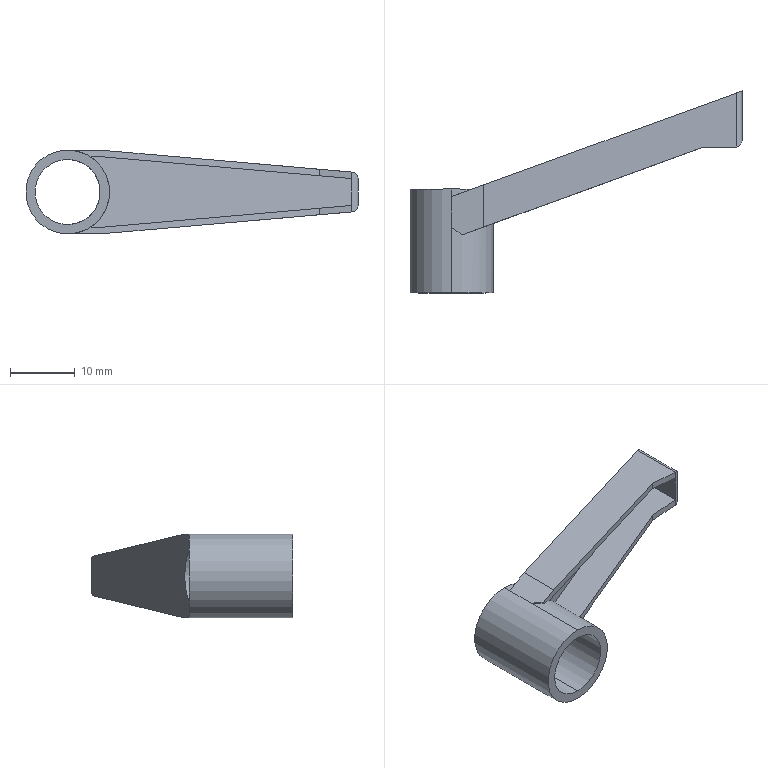Part | SolidWorks | features BaseBody 1, Shell 1 | 1 solid | 33 faces | box 51.5 x 31.3 x 13 mm | volume 1733 mm3 | plane 23 | cylinder 10 | commonest cylinder face diameters 13 x4 2 x3 10.1 x2 12.1 x1
STEP:
#1=CARTESIAN_POINT('',(3.238,20.3,5.636));
#2=VERTEX_POINT('',#1);
#3=CARTESIAN_POINT('',(0.,20.3,6.5));
#4=VERTEX_POINT('',#3);
#5=CARTESIAN_POINT('',(0.,20.3,0.));
#6=DIRECTION('',(0.,-1.,0.));
#7=DIRECTION('',(0.,0.,-1.));
#8=AXIS2_PLACEMENT_3D('',#5,#6,#7);
#9=CIRCLE('',#8,6.5);
#10=EDGE_CURVE('',#2,#4,#9,.T.);
#11=ORIENTED_EDGE('',*,*,#10,.T.);
#12=CARTESIAN_POINT('',(0.,19.121,6.5));
#13=VERTEX_POINT('',#12);
#14=CARTESIAN_POINT('',(0.,12.25,6.5));
#15=DIRECTION('',(0.,-1.,0.));
#16=VECTOR('',#15,1000.);
#17=LINE('',#14,#16);
#18=EDGE_CURVE('',#4,#13,#17,.T.);
#19=ORIENTED_EDGE('',*,*,#18,.T.);
#20=CARTESIAN_POINT('',(3.238,20.3,5.636));
#21=CARTESIAN_POINT('',(2.247,19.939,6.205));
#22=CARTESIAN_POINT('',(1.143,19.537,6.5));
#23=CARTESIAN_POINT('',(0.,19.121,6.5));
#24=(BOUNDED_CURVE()B_SPLINE_CURVE(3,(#20,#21,#22,#23),.UNSPECIFIED.,.F.,.F.)B_SPLINE_CURVE_WITH_KNOTS((4,4),(4.191,4.712),.UNSPECIFIED.)CURVE()GEOMETRIC_REPRESENTATION_ITEM()RATIONAL_B_SPLINE_CURVE((1.,0.9775,0.9775,1.))REPRESENTATION_ITEM(''));
#25=EDGE_CURVE('',#2,#13,#24,.T.);
#26=ORIENTED_EDGE('',*,*,#25,.F.);
#27=EDGE_LOOP('',(#11,#19,#26));
#28=FACE_OUTER_BOUND('',#27,.T.);
#29=CARTESIAN_POINT('',(0.,12.25,0.));
#30=DIRECTION('',(0.,-1.,0.));
#31=DIRECTION('',(0.,0.,-1.));
#32=AXIS2_PLACEMENT_3D('',#29,#30,#31);
#33=CYLINDRICAL_SURFACE('',#32,6.5);
#34=ADVANCED_FACE('',(#28),#33,.T.);
#35=CARTESIAN_POINT('',(1.638,13.2,6.29));
#36=VERTEX_POINT('',#35);
#37=CARTESIAN_POINT('',(0.,14.347,6.5));
#38=VERTEX_POINT('',#37);
#39=CARTESIAN_POINT('',(1.638,13.2,6.29));
#40=CARTESIAN_POINT('',(1.103,13.575,6.43));
#41=CARTESIAN_POINT('',(0.5536,13.959,6.5));
#42=CARTESIAN_POINT('',(0.,14.347,6.5));
#43=(BOUNDED_CURVE()B_SPLINE_CURVE(3,(#39,#40,#41,#42),.UNSPECIFIED.,.F.,.F.)B_SPLINE_CURVE_WITH_KNOTS((4,4),(1.316,1.571),.UNSPECIFIED.)CURVE()GEOMETRIC_REPRESENTATION_ITEM()RATIONAL_B_SPLINE_CURVE((1.,0.9946,0.9946,1.))REPRESENTATION_ITEM(''));
#44=EDGE_CURVE('',#36,#38,#43,.T.);
#45=ORIENTED_EDGE('',*,*,#44,.T.);
#46=CARTESIAN_POINT('',(0.,4.2,6.5));
#47=VERTEX_POINT('',#46);
#48=CARTESIAN_POINT('',(0.,12.25,6.5));
#49=DIRECTION('',(0.,-1.,0.));
#50=VECTOR('',#49,1000.);
#51=LINE('',#48,#50);
#52=EDGE_CURVE('',#38,#47,#51,.T.);
#53=ORIENTED_EDGE('',*,*,#52,.T.);
#54=CARTESIAN_POINT('',(0.,4.2,-6.5));
#55=VERTEX_POINT('',#54);
#56=CARTESIAN_POINT('',(0.,4.2,0.));
#57=DIRECTION('',(0.,1.,0.));
#58=DIRECTION('',(0.,0.,-1.));
#59=AXIS2_PLACEMENT_3D('',#56,#57,#58);
#60=CIRCLE('',#59,6.5);
#61=EDGE_CURVE('',#47,#55,#60,.T.);
#62=ORIENTED_EDGE('',*,*,#61,.T.);
#63=CARTESIAN_POINT('',(0.,14.347,-6.5));
#64=VERTEX_POINT('',#63);
#65=CARTESIAN_POINT('',(0.,12.25,-6.5));
#66=DIRECTION('',(0.,-1.,0.));
#67=VECTOR('',#66,1000.);
#68=LINE('',#65,#67);
#69=EDGE_CURVE('',#64,#55,#68,.T.);
#70=ORIENTED_EDGE('',*,*,#69,.F.);
#71=CARTESIAN_POINT('',(1.638,13.2,-6.29));
#72=VERTEX_POINT('',#71);
#73=CARTESIAN_POINT('',(0.,14.347,-6.5));
#74=CARTESIAN_POINT('',(0.5536,13.959,-6.5));
#75=CARTESIAN_POINT('',(1.103,13.575,-6.43));
#76=CARTESIAN_POINT('',(1.638,13.2,-6.29));
#77=(BOUNDED_CURVE()B_SPLINE_CURVE(3,(#73,#74,#75,#76),.UNSPECIFIED.,.F.,.T.)B_SPLINE_CURVE_WITH_KNOTS((4,4),(4.712,4.967),.UNSPECIFIED.)CURVE()GEOMETRIC_REPRESENTATION_ITEM()RATIONAL_B_SPLINE_CURVE((1.,0.9946,0.9946,1.))REPRESENTATION_ITEM(''));
#78=EDGE_CURVE('',#64,#72,#77,.T.);
#79=ORIENTED_EDGE('',*,*,#78,.T.);
#80=CARTESIAN_POINT('',(3.464,13.864,-5.5));
#81=VERTEX_POINT('',#80);
#82=CARTESIAN_POINT('',(1.638,13.2,-6.29));
#83=CARTESIAN_POINT('',(2.285,13.435,-6.122));
#84=CARTESIAN_POINT('',(2.899,13.658,-5.856));
#85=CARTESIAN_POINT('',(3.464,13.864,-5.5));
#86=(BOUNDED_CURVE()B_SPLINE_CURVE(3,(#82,#83,#84,#85),.UNSPECIFIED.,.F.,.T.)B_SPLINE_CURVE_WITH_KNOTS((4,4),(1.826,2.133),.UNSPECIFIED.)CURVE()GEOMETRIC_REPRESENTATION_ITEM()RATIONAL_B_SPLINE_CURVE((1.,0.9921,0.9921,1.))REPRESENTATION_ITEM(''));
#87=EDGE_CURVE('',#72,#81,#86,.T.);
#88=ORIENTED_EDGE('',*,*,#87,.T.);
#89=CARTESIAN_POINT('',(3.464,13.864,5.5));
#90=VERTEX_POINT('',#89);
#91=CARTESIAN_POINT('',(3.464,13.864,-5.5));
#92=CARTESIAN_POINT('',(7.97,15.504,-2.662));
#93=CARTESIAN_POINT('',(7.97,15.504,2.662));
#94=CARTESIAN_POINT('',(3.464,13.864,5.5));
#95=(BOUNDED_CURVE()B_SPLINE_CURVE(3,(#91,#92,#93,#94),.UNSPECIFIED.,.F.,.T.)B_SPLINE_CURVE_WITH_KNOTS((4,4),(2.133,4.15),.UNSPECIFIED.)CURVE()GEOMETRIC_REPRESENTATION_ITEM()RATIONAL_B_SPLINE_CURVE((1.,0.6886,0.6886,1.))REPRESENTATION_ITEM(''));
#96=EDGE_CURVE('',#81,#90,#95,.T.);
#97=ORIENTED_EDGE('',*,*,#96,.T.);
#98=CARTESIAN_POINT('',(3.464,13.864,5.5));
#99=CARTESIAN_POINT('',(2.899,13.658,5.856));
#100=CARTESIAN_POINT('',(2.285,13.435,6.122));
#101=CARTESIAN_POINT('',(1.638,13.2,6.29));
#102=(BOUNDED_CURVE()B_SPLINE_CURVE(3,(#98,#99,#100,#101),.UNSPECIFIED.,.F.,.F.)B_SPLINE_CURVE_WITH_KNOTS((4,4),(4.15,4.458),.UNSPECIFIED.)CURVE()GEOMETRIC_REPRESENTATION_ITEM()RATIONAL_B_SPLINE_CURVE((1.,0.9921,0.9921,1.))REPRESENTATION_ITEM(''));
#103=EDGE_CURVE('',#90,#36,#102,.T.);
#104=ORIENTED_EDGE('',*,*,#103,.T.);
#105=EDGE_LOOP('',(#45,#53,#62,#70,#79,#88,#97,#104));
#106=FACE_OUTER_BOUND('',#105,.T.);
#107=CARTESIAN_POINT('',(0.,12.25,0.));
#108=DIRECTION('',(0.,-1.,0.));
#109=DIRECTION('',(0.,0.,-1.));
#110=AXIS2_PLACEMENT_3D('',#107,#108,#109);
#111=CYLINDRICAL_SURFACE('',#110,6.5);
#112=ADVANCED_FACE('',(#106),#111,.T.);
#113=ORIENTED_EDGE('',*,*,#18,.F.);
#114=CARTESIAN_POINT('',(0.,20.3,-6.5));
#115=VERTEX_POINT('',#114);
#116=CARTESIAN_POINT('',(0.,20.3,0.));
#117=DIRECTION('',(0.,-1.,0.));
#118=DIRECTION('',(0.,0.,-1.));
#119=AXIS2_PLACEMENT_3D('',#116,#117,#118);
#120=CIRCLE('',#119,6.5);
#121=EDGE_CURVE('',#4,#115,#120,.T.);
#122=ORIENTED_EDGE('',*,*,#121,.T.);
#123=CARTESIAN_POINT('',(0.,19.121,-6.5));
#124=VERTEX_POINT('',#123);
#125=CARTESIAN_POINT('',(0.,12.25,-6.5));
#126=DIRECTION('',(0.,-1.,0.));
#127=VECTOR('',#126,1000.);
#128=LINE('',#125,#127);
#129=EDGE_CURVE('',#115,#124,#128,.T.);
#130=ORIENTED_EDGE('',*,*,#129,.T.);
#131=CARTESIAN_POINT('',(0.,12.25,-6.5));
#132=DIRECTION('',(0.,-1.,0.));
#133=VECTOR('',#132,1000.);
#134=LINE('',#131,#133);
#135=EDGE_CURVE('',#124,#64,#134,.T.);
#136=ORIENTED_EDGE('',*,*,#135,.T.);
#137=ORIENTED_EDGE('',*,*,#69,.T.);
#138=CARTESIAN_POINT('',(0.,4.2,0.));
#139=DIRECTION('',(0.,1.,0.));
#140=DIRECTION('',(0.,0.,-1.));
#141=AXIS2_PLACEMENT_3D('',#138,#139,#140);
#142=CIRCLE('',#141,6.5);
#143=EDGE_CURVE('',#55,#47,#142,.T.);
#144=ORIENTED_EDGE('',*,*,#143,.T.);
#145=ORIENTED_EDGE('',*,*,#52,.F.);
#146=CARTESIAN_POINT('',(0.,0.,6.5));
#147=DIRECTION('',(0.,-1.,0.));
#148=VECTOR('',#147,1000.);
#149=LINE('',#146,#148);
#150=EDGE_CURVE('',#13,#38,#149,.T.);
#151=ORIENTED_EDGE('',*,*,#150,.F.);
#152=EDGE_LOOP('',(#113,#122,#130,#136,#137,#144,#145,#151));
#153=FACE_OUTER_BOUND('',#152,.T.);
#154=CARTESIAN_POINT('',(0.,12.25,0.));
#155=DIRECTION('',(0.,-1.,0.));
#156=DIRECTION('',(0.,0.,-1.));
#157=AXIS2_PLACEMENT_3D('',#154,#155,#156);
#158=CYLINDRICAL_SURFACE('',#157,6.5);
#159=ADVANCED_FACE('',(#153),#158,.T.);
#160=CARTESIAN_POINT('',(0.,20.3,5.05));
#161=VERTEX_POINT('',#160);
#162=CARTESIAN_POINT('',(0.,20.3,-5.05));
#163=VERTEX_POINT('',#162);
#164=CARTESIAN_POINT('',(0.,20.3,0.));
#165=DIRECTION('',(0.,-1.,0.));
#166=DIRECTION('',(0.,0.,-1.));
#167=AXIS2_PLACEMENT_3D('',#164,#165,#166);
#168=CIRCLE('',#167,5.05);
#169=EDGE_CURVE('',#161,#163,#168,.T.);
#170=ORIENTED_EDGE('',*,*,#169,.F.);
#171=CARTESIAN_POINT('',(0.,4.2,5.05));
#172=VERTEX_POINT('',#171);
#173=CARTESIAN_POINT('',(0.,14.35,5.05));
#174=DIRECTION('',(0.,-1.,0.));
#175=VECTOR('',#174,1000.);
#176=LINE('',#173,#175);
#177=EDGE_CURVE('',#161,#172,#176,.T.);
#178=ORIENTED_EDGE('',*,*,#177,.T.);
#179=CARTESIAN_POINT('',(0.,4.2,-5.05));
#180=VERTEX_POINT('',#179);
#181=CARTESIAN_POINT('',(0.,4.2,0.));
#182=DIRECTION('',(0.,1.,0.));
#183=DIRECTION('',(0.,0.,-1.));
#184=AXIS2_PLACEMENT_3D('',#181,#182,#183);
#185=CIRCLE('',#184,5.05);
#186=EDGE_CURVE('',#180,#172,#185,.T.);
#187=ORIENTED_EDGE('',*,*,#186,.F.);
#188=CARTESIAN_POINT('',(0.,14.35,-5.05));
#189=DIRECTION('',(0.,-1.,0.));
#190=VECTOR('',#189,1000.);
#191=LINE('',#188,#190);
#192=EDGE_CURVE('',#163,#180,#191,.T.);
#193=ORIENTED_EDGE('',*,*,#192,.F.);
#194=EDGE_LOOP('',(#170,#178,#187,#193));
#195=FACE_OUTER_BOUND('',#194,.T.);
#196=CARTESIAN_POINT('',(0.,14.35,0.));
#197=DIRECTION('',(0.,-1.,0.));
#198=DIRECTION('',(0.,0.,-1.));
#199=AXIS2_PLACEMENT_3D('',#196,#197,#198);
#200=CYLINDRICAL_SURFACE('',#199,5.05);
#201=ADVANCED_FACE('',(#195),#200,.F.);
#202=CARTESIAN_POINT('',(39.031,26.809,-2.519));
#203=VERTEX_POINT('',#202);
#204=CARTESIAN_POINT('',(44.,26.809,-2.084));
#205=VERTEX_POINT('',#204);
#206=CARTESIAN_POINT('',(44.,26.809,-2.084));
#207=DIRECTION('',(0.9962,0.,0.08716));
#208=VECTOR('',#207,1000.);
#209=LINE('',#206,#208);
#210=EDGE_CURVE('',#203,#205,#209,.T.);
#211=ORIENTED_EDGE('',*,*,#210,.F.);
#212=CARTESIAN_POINT('',(39.031,26.809,-3.523));
#213=VERTEX_POINT('',#212);
#214=CARTESIAN_POINT('',(39.031,26.809,6.5));
#215=DIRECTION('',(0.,0.,1.));
#216=VECTOR('',#215,1000.);
#217=LINE('',#214,#216);
#218=EDGE_CURVE('',#213,#203,#217,.T.);
#219=ORIENTED_EDGE('',*,*,#218,.F.);
#220=CARTESIAN_POINT('',(44.,26.809,-3.088));
#221=VERTEX_POINT('',#220);
#222=CARTESIAN_POINT('',(44.087,26.809,-3.08));
#223=DIRECTION('',(0.9962,0.,0.08716));
#224=VECTOR('',#223,1000.);
#225=LINE('',#222,#224);
#226=EDGE_CURVE('',#213,#221,#225,.T.);
#227=ORIENTED_EDGE('',*,*,#226,.T.);
#228=CARTESIAN_POINT('',(44.,26.809,6.5));
#229=DIRECTION('',(0.,0.,1.));
#230=VECTOR('',#229,1000.);
#231=LINE('',#228,#230);
#232=EDGE_CURVE('',#221,#205,#231,.T.);
#233=ORIENTED_EDGE('',*,*,#232,.T.);
#234=EDGE_LOOP('',(#211,#219,#227,#233));
#235=FACE_OUTER_BOUND('',#234,.T.);
#236=CARTESIAN_POINT('',(39.031,26.809,6.5));
#237=DIRECTION('',(0.,-1.,0.));
#238=DIRECTION('',(0.,0.,-1.));
#239=AXIS2_PLACEMENT_3D('',#236,#237,#238);
#240=PLANE('',#239);
#241=ADVANCED_FACE('',(#235),#240,.T.);
#242=CARTESIAN_POINT('',(4.956,14.407,-5.5));
#243=VERTEX_POINT('',#242);
#244=CARTESIAN_POINT('',(-4.051,11.129,-5.5));
#245=DIRECTION('',(0.9397,0.342,0.));
#246=VECTOR('',#245,1000.);
#247=LINE('',#244,#246);
#248=EDGE_CURVE('',#81,#243,#247,.T.);
#249=ORIENTED_EDGE('',*,*,#248,.F.);
#250=ORIENTED_EDGE('',*,*,#87,.F.);
#251=CARTESIAN_POINT('',(1.638,13.2,-6.5));
#252=VERTEX_POINT('',#251);
#253=CARTESIAN_POINT('',(1.638,13.2,6.5));
#254=DIRECTION('',(0.,0.,-1.));
#255=VECTOR('',#254,1000.);
#256=LINE('',#253,#255);
#257=EDGE_CURVE('',#72,#252,#256,.T.);
#258=ORIENTED_EDGE('',*,*,#257,.T.);
#259=CARTESIAN_POINT('',(5.,14.423,-6.5));
#260=VERTEX_POINT('',#259);
#261=CARTESIAN_POINT('',(1.638,13.2,-6.5));
#262=DIRECTION('',(0.9397,0.342,0.));
#263=VECTOR('',#262,1000.);
#264=LINE('',#261,#263);
#265=EDGE_CURVE('',#252,#260,#264,.T.);
#266=ORIENTED_EDGE('',*,*,#265,.T.);
#267=CARTESIAN_POINT('',(5.,14.423,-6.5));
#268=DIRECTION('',(0.9365,0.3409,0.08194));
#269=VECTOR('',#268,1000.);
#270=LINE('',#267,#269);
#271=EDGE_CURVE('',#260,#213,#270,.T.);
#272=ORIENTED_EDGE('',*,*,#271,.T.);
#273=ORIENTED_EDGE('',*,*,#218,.T.);
#274=CARTESIAN_POINT('',(38.775,26.716,-2.541));
#275=DIRECTION('',(0.9365,0.3409,0.08194));
#276=VECTOR('',#275,1000.);
#277=LINE('',#274,#276);
#278=EDGE_CURVE('',#243,#203,#277,.T.);
#279=ORIENTED_EDGE('',*,*,#278,.F.);
#280=EDGE_LOOP('',(#249,#250,#258,#266,#272,#273,#279));
#281=FACE_OUTER_BOUND('',#280,.T.);
#282=CARTESIAN_POINT('',(1.638,13.2,6.5));
#283=DIRECTION('',(0.342,-0.9397,0.));
#284=DIRECTION('',(0.9397,0.342,0.));
#285=AXIS2_PLACEMENT_3D('',#282,#283,#284);
#286=PLANE('',#285);
#287=ADVANCED_FACE('',(#281),#286,.T.);
#288=ORIENTED_EDGE('',*,*,#25,.T.);
#289=CARTESIAN_POINT('',(5.,20.941,6.5));
#290=VERTEX_POINT('',#289);
#291=CARTESIAN_POINT('',(45.,35.5,6.5));
#292=DIRECTION('',(0.9397,0.342,0.));
#293=VECTOR('',#292,1000.);
#294=LINE('',#291,#293);
#295=EDGE_CURVE('',#13,#290,#294,.T.);
#296=ORIENTED_EDGE('',*,*,#295,.T.);
#297=CARTESIAN_POINT('',(44.087,35.168,3.08));
#298=VERTEX_POINT('',#297);
#299=CARTESIAN_POINT('',(5.,20.941,6.5));
#300=DIRECTION('',(0.9365,0.3409,-0.08194));
#301=VECTOR('',#300,1000.);
#302=LINE('',#299,#301);
#303=EDGE_CURVE('',#290,#298,#302,.T.);
#304=ORIENTED_EDGE('',*,*,#303,.T.);
#305=CARTESIAN_POINT('',(45.,35.5,2.084));
#306=VERTEX_POINT('',#305);
#307=CARTESIAN_POINT('',(45.,35.5,2.084));
#308=CARTESIAN_POINT('',(45.,35.5,2.63));
#309=CARTESIAN_POINT('',(44.631,35.366,3.033));
#310=CARTESIAN_POINT('',(44.087,35.168,3.08));
#311=(BOUNDED_CURVE()B_SPLINE_CURVE(3,(#307,#308,#309,#310),.UNSPECIFIED.,.F.,.F.)B_SPLINE_CURVE_WITH_KNOTS((4,4),(3.142,4.625),.UNSPECIFIED.)CURVE()GEOMETRIC_REPRESENTATION_ITEM()RATIONAL_B_SPLINE_CURVE((1.,0.8249,0.8249,1.))REPRESENTATION_ITEM(''));
#312=EDGE_CURVE('',#306,#298,#311,.T.);
#313=ORIENTED_EDGE('',*,*,#312,.F.);
#314=CARTESIAN_POINT('',(45.,35.5,-2.084));
#315=VERTEX_POINT('',#314);
#316=CARTESIAN_POINT('',(45.,35.5,6.5));
#317=DIRECTION('',(0.,0.,-1.));
#318=VECTOR('',#317,1000.);
#319=LINE('',#316,#318);
#320=EDGE_CURVE('',#306,#315,#319,.T.);
#321=ORIENTED_EDGE('',*,*,#320,.T.);
#322=CARTESIAN_POINT('',(44.087,35.168,-3.08));
#323=VERTEX_POINT('',#322);
#324=CARTESIAN_POINT('',(44.087,35.168,-3.08));
#325=CARTESIAN_POINT('',(44.631,35.366,-3.033));
#326=CARTESIAN_POINT('',(45.,35.5,-2.63));
#327=CARTESIAN_POINT('',(45.,35.5,-2.084));
#328=(BOUNDED_CURVE()B_SPLINE_CURVE(3,(#324,#325,#326,#327),.UNSPECIFIED.,.F.,.F.)B_SPLINE_CURVE_WITH_KNOTS((4,4),(1.658,3.142),.UNSPECIFIED.)CURVE()GEOMETRIC_REPRESENTATION_ITEM()RATIONAL_B_SPLINE_CURVE((1.,0.8249,0.8249,1.))REPRESENTATION_ITEM(''));
#329=EDGE_CURVE('',#323,#315,#328,.T.);
#330=ORIENTED_EDGE('',*,*,#329,.F.);
#331=CARTESIAN_POINT('',(5.,20.941,-6.5));
#332=VERTEX_POINT('',#331);
#333=CARTESIAN_POINT('',(44.087,35.168,-3.08));
#334=DIRECTION('',(-0.9365,-0.3409,-0.08194));
#335=VECTOR('',#334,1000.);
#336=LINE('',#333,#335);
#337=EDGE_CURVE('',#323,#332,#336,.T.);
#338=ORIENTED_EDGE('',*,*,#337,.T.);
#339=CARTESIAN_POINT('',(45.,35.5,-6.5));
#340=DIRECTION('',(-0.9397,-0.342,0.));
#341=VECTOR('',#340,1000.);
#342=LINE('',#339,#341);
#343=EDGE_CURVE('',#332,#124,#342,.T.);
#344=ORIENTED_EDGE('',*,*,#343,.T.);
#345=CARTESIAN_POINT('',(3.238,20.3,-5.636));
#346=VERTEX_POINT('',#345);
#347=CARTESIAN_POINT('',(0.,19.121,-6.5));
#348=CARTESIAN_POINT('',(1.143,19.537,-6.5));
#349=CARTESIAN_POINT('',(2.247,19.939,-6.205));
#350=CARTESIAN_POINT('',(3.238,20.3,-5.636));
#351=(BOUNDED_CURVE()B_SPLINE_CURVE(3,(#347,#348,#349,#350),.UNSPECIFIED.,.F.,.T.)B_SPLINE_CURVE_WITH_KNOTS((4,4),(1.571,2.092),.UNSPECIFIED.)CURVE()GEOMETRIC_REPRESENTATION_ITEM()RATIONAL_B_SPLINE_CURVE((1.,0.9775,0.9775,1.))REPRESENTATION_ITEM(''));
#352=EDGE_CURVE('',#124,#346,#351,.T.);
#353=ORIENTED_EDGE('',*,*,#352,.T.);
#354=CARTESIAN_POINT('',(3.238,20.3,-3.875));
#355=VERTEX_POINT('',#354);
#356=CARTESIAN_POINT('',(3.238,20.3,6.5));
#357=DIRECTION('',(0.,0.,1.));
#358=VECTOR('',#357,1000.);
#359=LINE('',#356,#358);
#360=EDGE_CURVE('',#346,#355,#359,.T.);
#361=ORIENTED_EDGE('',*,*,#360,.T.);
#362=CARTESIAN_POINT('',(3.238,20.3,3.875));
#363=VERTEX_POINT('',#362);
#364=CARTESIAN_POINT('',(3.238,20.3,-3.875));
#365=CARTESIAN_POINT('',(5.844,21.248,-1.698));
#366=CARTESIAN_POINT('',(5.844,21.248,1.698));
#367=CARTESIAN_POINT('',(3.238,20.3,3.875));
#368=(BOUNDED_CURVE()B_SPLINE_CURVE(3,(#364,#365,#366,#367),.UNSPECIFIED.,.F.,.F.)B_SPLINE_CURVE_WITH_KNOTS((4,4),(2.267,4.016),.UNSPECIFIED.)CURVE()GEOMETRIC_REPRESENTATION_ITEM()RATIONAL_B_SPLINE_CURVE((1.,0.7608,0.7608,1.))REPRESENTATION_ITEM(''));
#369=EDGE_CURVE('',#355,#363,#368,.T.);
#370=ORIENTED_EDGE('',*,*,#369,.T.);
#371=CARTESIAN_POINT('',(3.238,20.3,6.5));
#372=DIRECTION('',(0.,0.,1.));
#373=VECTOR('',#372,1000.);
#374=LINE('',#371,#373);
#375=EDGE_CURVE('',#363,#2,#374,.T.);
#376=ORIENTED_EDGE('',*,*,#375,.T.);
#377=EDGE_LOOP('',(#288,#296,#304,#313,#321,#330,#338,#344,#353,#361,#370,#376));
#378=FACE_OUTER_BOUND('',#377,.T.);
#379=CARTESIAN_POINT('',(45.,35.5,6.5));
#380=DIRECTION('',(-0.342,0.9397,0.));
#381=DIRECTION('',(-0.9397,-0.342,0.));
#382=AXIS2_PLACEMENT_3D('',#379,#380,#381);
#383=PLANE('',#382);
#384=ADVANCED_FACE('',(#378),#383,.T.);
#385=CARTESIAN_POINT('',(1.638,13.2,6.5));
#386=VERTEX_POINT('',#385);
#387=CARTESIAN_POINT('',(0.,14.347,6.5));
#388=DIRECTION('',(0.8192,-0.5736,0.));
#389=VECTOR('',#388,1000.);
#390=LINE('',#387,#389);
#391=EDGE_CURVE('',#38,#386,#390,.T.);
#392=ORIENTED_EDGE('',*,*,#391,.T.);
#393=CARTESIAN_POINT('',(5.,14.423,6.5));
#394=VERTEX_POINT('',#393);
#395=CARTESIAN_POINT('',(1.638,13.2,6.5));
#396=DIRECTION('',(0.9397,0.342,0.));
#397=VECTOR('',#396,1000.);
#398=LINE('',#395,#397);
#399=EDGE_CURVE('',#386,#394,#398,.T.);
#400=ORIENTED_EDGE('',*,*,#399,.T.);
#401=CARTESIAN_POINT('',(5.,0.,6.5));
#402=DIRECTION('',(0.,1.,0.));
#403=VECTOR('',#402,1000.);
#404=LINE('',#401,#403);
#405=EDGE_CURVE('',#394,#290,#404,.T.);
#406=ORIENTED_EDGE('',*,*,#405,.T.);
#407=ORIENTED_EDGE('',*,*,#295,.F.);
#408=ORIENTED_EDGE('',*,*,#150,.T.);
#409=EDGE_LOOP('',(#392,#400,#406,#407,#408));
#410=FACE_OUTER_BOUND('',#409,.T.);
#411=CARTESIAN_POINT('',(0.,0.,6.5));
#412=DIRECTION('',(0.,0.,1.));
#413=DIRECTION('',(1.,0.,0.));
#414=AXIS2_PLACEMENT_3D('',#411,#412,#413);
#415=PLANE('',#414);
#416=ADVANCED_FACE('',(#410),#415,.T.);
#417=ORIENTED_EDGE('',*,*,#129,.F.);
#418=CARTESIAN_POINT('',(0.,20.3,0.));
#419=DIRECTION('',(0.,-1.,0.));
#420=DIRECTION('',(0.,0.,-1.));
#421=AXIS2_PLACEMENT_3D('',#418,#419,#420);
#422=CIRCLE('',#421,6.5);
#423=EDGE_CURVE('',#115,#346,#422,.T.);
#424=ORIENTED_EDGE('',*,*,#423,.T.);
#425=ORIENTED_EDGE('',*,*,#352,.F.);
#426=EDGE_LOOP('',(#417,#424,#425));
#427=FACE_OUTER_BOUND('',#426,.T.);
#428=CARTESIAN_POINT('',(0.,12.25,0.));
#429=DIRECTION('',(0.,-1.,0.));
#430=DIRECTION('',(0.,0.,-1.));
#431=AXIS2_PLACEMENT_3D('',#428,#429,#430);
#432=CYLINDRICAL_SURFACE('',#431,6.5);
#433=ADVANCED_FACE('',(#427),#432,.T.);
#434=ORIENTED_EDGE('',*,*,#10,.F.);
#435=ORIENTED_EDGE('',*,*,#375,.F.);
#436=CARTESIAN_POINT('',(0.,20.3,0.));
#437=DIRECTION('',(0.,-1.,0.));
#438=DIRECTION('',(0.,0.,-1.));
#439=AXIS2_PLACEMENT_3D('',#436,#437,#438);
#440=CIRCLE('',#439,5.05);
#441=EDGE_CURVE('',#363,#161,#440,.T.);
#442=ORIENTED_EDGE('',*,*,#441,.T.);
#443=ORIENTED_EDGE('',*,*,#169,.T.);
#444=CARTESIAN_POINT('',(0.,20.3,0.));
#445=DIRECTION('',(0.,-1.,0.));
#446=DIRECTION('',(0.,0.,-1.));
#447=AXIS2_PLACEMENT_3D('',#444,#445,#446);
#448=CIRCLE('',#447,5.05);
#449=EDGE_CURVE('',#163,#355,#448,.T.);
#450=ORIENTED_EDGE('',*,*,#449,.T.);
#451=ORIENTED_EDGE('',*,*,#360,.F.);
#452=ORIENTED_EDGE('',*,*,#423,.F.);
#453=ORIENTED_EDGE('',*,*,#121,.F.);
#454=EDGE_LOOP('',(#434,#435,#442,#443,#450,#451,#452,#453));
#455=FACE_OUTER_BOUND('',#454,.T.);
#456=CARTESIAN_POINT('',(3.25,20.3,0.));
#457=DIRECTION('',(0.,1.,0.));
#458=DIRECTION('',(0.,0.,1.));
#459=AXIS2_PLACEMENT_3D('',#456,#457,#458);
#460=PLANE('',#459);
#461=ADVANCED_FACE('',(#455),#460,.T.);
#462=ORIENTED_EDGE('',*,*,#177,.F.);
#463=ORIENTED_EDGE('',*,*,#441,.F.);
#464=ORIENTED_EDGE('',*,*,#369,.F.);
#465=ORIENTED_EDGE('',*,*,#449,.F.);
#466=ORIENTED_EDGE('',*,*,#192,.T.);
#467=CARTESIAN_POINT('',(0.,4.2,0.));
#468=DIRECTION('',(0.,1.,0.));
#469=DIRECTION('',(0.,0.,-1.));
#470=AXIS2_PLACEMENT_3D('',#467,#468,#469);
#471=CIRCLE('',#470,5.05);
#472=EDGE_CURVE('',#172,#180,#471,.T.);
#473=ORIENTED_EDGE('',*,*,#472,.F.);
#474=EDGE_LOOP('',(#462,#463,#464,#465,#466,#473));
#475=FACE_OUTER_BOUND('',#474,.T.);
#476=CARTESIAN_POINT('',(0.,14.35,0.));
#477=DIRECTION('',(0.,-1.,0.));
#478=DIRECTION('',(0.,0.,-1.));
#479=AXIS2_PLACEMENT_3D('',#476,#477,#478);
#480=CYLINDRICAL_SURFACE('',#479,5.05);
#481=ADVANCED_FACE('',(#475),#480,.F.);
#482=ORIENTED_EDGE('',*,*,#265,.F.);
#483=CARTESIAN_POINT('',(0.,14.347,-6.5));
#484=DIRECTION('',(0.8192,-0.5736,0.));
#485=VECTOR('',#484,1000.);
#486=LINE('',#483,#485);
#487=EDGE_CURVE('',#64,#252,#486,.T.);
#488=ORIENTED_EDGE('',*,*,#487,.F.);
#489=ORIENTED_EDGE('',*,*,#135,.F.);
#490=ORIENTED_EDGE('',*,*,#343,.F.);
#491=CARTESIAN_POINT('',(5.,0.,-6.5));
#492=DIRECTION('',(0.,1.,0.));
#493=VECTOR('',#492,1000.);
#494=LINE('',#491,#493);
#495=EDGE_CURVE('',#260,#332,#494,.T.);
#496=ORIENTED_EDGE('',*,*,#495,.F.);
#497=EDGE_LOOP('',(#482,#488,#489,#490,#496));
#498=FACE_OUTER_BOUND('',#497,.T.);
#499=CARTESIAN_POINT('',(0.,0.,-6.5));
#500=DIRECTION('',(0.,0.,1.));
#501=DIRECTION('',(1.,0.,0.));
#502=AXIS2_PLACEMENT_3D('',#499,#500,#501);
#503=PLANE('',#502);
#504=ADVANCED_FACE('',(#498),#503,.F.);
#505=ORIENTED_EDGE('',*,*,#226,.F.);
#506=ORIENTED_EDGE('',*,*,#271,.F.);
#507=ORIENTED_EDGE('',*,*,#495,.T.);
#508=ORIENTED_EDGE('',*,*,#337,.F.);
#509=CARTESIAN_POINT('',(44.087,26.813,-3.08));
#510=VERTEX_POINT('',#509);
#511=CARTESIAN_POINT('',(44.087,12.25,-3.08));
#512=DIRECTION('',(0.,1.,0.));
#513=VECTOR('',#512,1000.);
#514=LINE('',#511,#513);
#515=EDGE_CURVE('',#510,#323,#514,.T.);
#516=ORIENTED_EDGE('',*,*,#515,.F.);
#517=CARTESIAN_POINT('',(44.,26.809,-3.088));
#518=CARTESIAN_POINT('',(44.029,26.809,-3.085));
#519=CARTESIAN_POINT('',(44.058,26.81,-3.083));
#520=CARTESIAN_POINT('',(44.087,26.813,-3.08));
#521=(BOUNDED_CURVE()B_SPLINE_CURVE(3,(#517,#518,#519,#520),.UNSPECIFIED.,.F.,.F.)B_SPLINE_CURVE_WITH_KNOTS((4,4),(4.712,4.8),.UNSPECIFIED.)CURVE()GEOMETRIC_REPRESENTATION_ITEM()RATIONAL_B_SPLINE_CURVE((1.,0.9994,0.9994,1.))REPRESENTATION_ITEM(''));
#522=EDGE_CURVE('',#221,#510,#521,.T.);
#523=ORIENTED_EDGE('',*,*,#522,.F.);
#524=EDGE_LOOP('',(#505,#506,#507,#508,#516,#523));
#525=FACE_OUTER_BOUND('',#524,.T.);
#526=CARTESIAN_POINT('',(44.087,12.25,-3.08));
#527=DIRECTION('',(-0.08716,0.,0.9962));
#528=DIRECTION('',(0.9962,0.,0.08716));
#529=AXIS2_PLACEMENT_3D('',#526,#527,#528);
#530=PLANE('',#529);
#531=ADVANCED_FACE('',(#525),#530,.F.);
#532=CARTESIAN_POINT('',(45.,27.809,-2.084));
#533=VERTEX_POINT('',#532);
#534=CARTESIAN_POINT('',(45.,27.809,-2.084));
#535=DIRECTION('',(0.,1.,0.));
#536=VECTOR('',#535,1000.);
#537=LINE('',#534,#536);
#538=EDGE_CURVE('',#533,#315,#537,.T.);
#539=ORIENTED_EDGE('',*,*,#538,.T.);
#540=ORIENTED_EDGE('',*,*,#320,.F.);
#541=CARTESIAN_POINT('',(45.,27.809,2.084));
#542=VERTEX_POINT('',#541);
#543=CARTESIAN_POINT('',(45.,27.809,2.084));
#544=DIRECTION('',(0.,-1.,0.));
#545=VECTOR('',#544,1000.);
#546=LINE('',#543,#545);
#547=EDGE_CURVE('',#306,#542,#546,.T.);
#548=ORIENTED_EDGE('',*,*,#547,.T.);
#549=CARTESIAN_POINT('',(45.,27.809,6.5));
#550=DIRECTION('',(0.,0.,-1.));
#551=VECTOR('',#550,1000.);
#552=LINE('',#549,#551);
#553=EDGE_CURVE('',#542,#533,#552,.T.);
#554=ORIENTED_EDGE('',*,*,#553,.T.);
#555=EDGE_LOOP('',(#539,#540,#548,#554));
#556=FACE_OUTER_BOUND('',#555,.T.);
#557=CARTESIAN_POINT('',(45.,27.809,6.5));
#558=DIRECTION('',(1.,0.,0.));
#559=DIRECTION('',(0.,0.,-1.));
#560=AXIS2_PLACEMENT_3D('',#557,#558,#559);
#561=PLANE('',#560);
#562=ADVANCED_FACE('',(#556),#561,.T.);
#563=CARTESIAN_POINT('',(44.,26.809,3.088));
#564=VERTEX_POINT('',#563);
#565=CARTESIAN_POINT('',(39.031,26.809,3.523));
#566=VERTEX_POINT('',#565);
#567=CARTESIAN_POINT('',(5.,26.809,6.5));
#568=DIRECTION('',(-0.9962,0.,0.08716));
#569=VECTOR('',#568,1000.);
#570=LINE('',#567,#569);
#571=EDGE_CURVE('',#564,#566,#570,.T.);
#572=ORIENTED_EDGE('',*,*,#571,.F.);
#573=CARTESIAN_POINT('',(44.087,26.813,3.08));
#574=VERTEX_POINT('',#573);
#575=CARTESIAN_POINT('',(44.087,26.813,3.08));
#576=CARTESIAN_POINT('',(44.058,26.81,3.083));
#577=CARTESIAN_POINT('',(44.029,26.809,3.085));
#578=CARTESIAN_POINT('',(44.,26.809,3.088));
#579=(BOUNDED_CURVE()B_SPLINE_CURVE(3,(#575,#576,#577,#578),.UNSPECIFIED.,.F.,.F.)B_SPLINE_CURVE_WITH_KNOTS((4,4),(4.625,4.712),.UNSPECIFIED.)CURVE()GEOMETRIC_REPRESENTATION_ITEM()RATIONAL_B_SPLINE_CURVE((1.,0.9994,0.9994,1.))REPRESENTATION_ITEM(''));
#580=EDGE_CURVE('',#574,#564,#579,.T.);
#581=ORIENTED_EDGE('',*,*,#580,.F.);
#582=CARTESIAN_POINT('',(44.087,12.25,3.08));
#583=DIRECTION('',(0.,-1.,0.));
#584=VECTOR('',#583,1000.);
#585=LINE('',#582,#584);
#586=EDGE_CURVE('',#298,#574,#585,.T.);
#587=ORIENTED_EDGE('',*,*,#586,.F.);
#588=ORIENTED_EDGE('',*,*,#303,.F.);
#589=ORIENTED_EDGE('',*,*,#405,.F.);
#590=CARTESIAN_POINT('',(39.031,26.809,3.523));
#591=DIRECTION('',(-0.9365,-0.3409,0.08194));
#592=VECTOR('',#591,1000.);
#593=LINE('',#590,#592);
#594=EDGE_CURVE('',#566,#394,#593,.T.);
#595=ORIENTED_EDGE('',*,*,#594,.F.);
#596=EDGE_LOOP('',(#572,#581,#587,#588,#589,#595));
#597=FACE_OUTER_BOUND('',#596,.T.);
#598=CARTESIAN_POINT('',(5.,12.25,6.5));
#599=DIRECTION('',(-0.08716,0.,-0.9962));
#600=DIRECTION('',(-0.9962,0.,0.08716));
#601=AXIS2_PLACEMENT_3D('',#598,#599,#600);
#602=PLANE('',#601);
#603=ADVANCED_FACE('',(#597),#602,.F.);
#604=CARTESIAN_POINT('',(39.031,26.809,2.519));
#605=VERTEX_POINT('',#604);
#606=CARTESIAN_POINT('',(4.956,14.407,5.5));
#607=VERTEX_POINT('',#606);
#608=CARTESIAN_POINT('',(4.229,14.143,5.564));
#609=DIRECTION('',(-0.9365,-0.3409,0.08194));
#610=VECTOR('',#609,1000.);
#611=LINE('',#608,#610);
#612=EDGE_CURVE('',#605,#607,#611,.T.);
#613=ORIENTED_EDGE('',*,*,#612,.F.);
#614=CARTESIAN_POINT('',(39.031,26.809,6.5));
#615=DIRECTION('',(0.,0.,1.));
#616=VECTOR('',#615,1000.);
#617=LINE('',#614,#616);
#618=EDGE_CURVE('',#605,#566,#617,.T.);
#619=ORIENTED_EDGE('',*,*,#618,.T.);
#620=ORIENTED_EDGE('',*,*,#594,.T.);
#621=ORIENTED_EDGE('',*,*,#399,.F.);
#622=CARTESIAN_POINT('',(1.638,13.2,6.5));
#623=DIRECTION('',(0.,0.,-1.));
#624=VECTOR('',#623,1000.);
#625=LINE('',#622,#624);
#626=EDGE_CURVE('',#386,#36,#625,.T.);
#627=ORIENTED_EDGE('',*,*,#626,.T.);
#628=ORIENTED_EDGE('',*,*,#103,.F.);
#629=CARTESIAN_POINT('',(-4.051,11.129,5.5));
#630=DIRECTION('',(0.9397,0.342,0.));
#631=VECTOR('',#630,1000.);
#632=LINE('',#629,#631);
#633=EDGE_CURVE('',#90,#607,#632,.T.);
#634=ORIENTED_EDGE('',*,*,#633,.T.);
#635=EDGE_LOOP('',(#613,#619,#620,#621,#627,#628,#634));
#636=FACE_OUTER_BOUND('',#635,.T.);
#637=CARTESIAN_POINT('',(1.638,13.2,6.5));
#638=DIRECTION('',(0.342,-0.9397,0.));
#639=DIRECTION('',(0.9397,0.342,0.));
#640=AXIS2_PLACEMENT_3D('',#637,#638,#639);
#641=PLANE('',#640);
#642=ADVANCED_FACE('',(#636),#641,.T.);
#643=ORIENTED_EDGE('',*,*,#626,.F.);
#644=ORIENTED_EDGE('',*,*,#391,.F.);
#645=ORIENTED_EDGE('',*,*,#44,.F.);
#646=EDGE_LOOP('',(#643,#644,#645));
#647=FACE_OUTER_BOUND('',#646,.T.);
#648=CARTESIAN_POINT('',(0.,14.347,6.5));
#649=DIRECTION('',(-0.5736,-0.8192,0.));
#650=DIRECTION('',(0.8192,-0.5736,0.));
#651=AXIS2_PLACEMENT_3D('',#648,#649,#650);
#652=PLANE('',#651);
#653=ADVANCED_FACE('',(#647),#652,.T.);
#654=ORIENTED_EDGE('',*,*,#143,.F.);
#655=ORIENTED_EDGE('',*,*,#61,.F.);
#656=EDGE_LOOP('',(#654,#655));
#657=FACE_OUTER_BOUND('',#656,.T.);
#658=ORIENTED_EDGE('',*,*,#186,.T.);
#659=ORIENTED_EDGE('',*,*,#472,.T.);
#660=EDGE_LOOP('',(#658,#659));
#661=FACE_BOUND('',#660,.T.);
#662=CARTESIAN_POINT('',(3.25,4.2,0.));
#663=DIRECTION('',(0.,-1.,0.));
#664=DIRECTION('',(1.,0.,0.));
#665=AXIS2_PLACEMENT_3D('',#662,#663,#664);
#666=PLANE('',#665);
#667=ADVANCED_FACE('',(#657,#661),#666,.T.);
#668=ORIENTED_EDGE('',*,*,#487,.T.);
#669=ORIENTED_EDGE('',*,*,#257,.F.);
#670=ORIENTED_EDGE('',*,*,#78,.F.);
#671=EDGE_LOOP('',(#668,#669,#670));
#672=FACE_OUTER_BOUND('',#671,.T.);
#673=CARTESIAN_POINT('',(0.,14.347,6.5));
#674=DIRECTION('',(-0.5736,-0.8192,0.));
#675=DIRECTION('',(0.8192,-0.5736,0.));
#676=AXIS2_PLACEMENT_3D('',#673,#674,#675);
#677=PLANE('',#676);
#678=ADVANCED_FACE('',(#672),#677,.T.);
#679=CARTESIAN_POINT('',(44.,26.809,2.084));
#680=VERTEX_POINT('',#679);
#681=CARTESIAN_POINT('',(4.913,26.809,5.504));
#682=DIRECTION('',(-0.9962,0.,0.08716));
#683=VECTOR('',#682,1000.);
#684=LINE('',#681,#683);
#685=EDGE_CURVE('',#680,#605,#684,.T.);
#686=ORIENTED_EDGE('',*,*,#685,.F.);
#687=CARTESIAN_POINT('',(44.,26.809,6.5));
#688=DIRECTION('',(0.,0.,1.));
#689=VECTOR('',#688,1000.);
#690=LINE('',#687,#689);
#691=EDGE_CURVE('',#680,#564,#690,.T.);
#692=ORIENTED_EDGE('',*,*,#691,.T.);
#693=ORIENTED_EDGE('',*,*,#571,.T.);
#694=ORIENTED_EDGE('',*,*,#618,.F.);
#695=EDGE_LOOP('',(#686,#692,#693,#694));
#696=FACE_OUTER_BOUND('',#695,.T.);
#697=CARTESIAN_POINT('',(39.031,26.809,6.5));
#698=DIRECTION('',(0.,-1.,0.));
#699=DIRECTION('',(0.,0.,-1.));
#700=AXIS2_PLACEMENT_3D('',#697,#698,#699);
#701=PLANE('',#700);
#702=ADVANCED_FACE('',(#696),#701,.T.);
#703=ORIENTED_EDGE('',*,*,#329,.T.);
#704=ORIENTED_EDGE('',*,*,#538,.F.);
#705=CARTESIAN_POINT('',(45.,27.809,-2.084));
#706=CARTESIAN_POINT('',(45.,27.263,-2.63));
#707=CARTESIAN_POINT('',(44.631,26.861,-3.033));
#708=CARTESIAN_POINT('',(44.087,26.813,-3.08));
#709=(BOUNDED_CURVE()B_SPLINE_CURVE(3,(#705,#706,#707,#708),.UNSPECIFIED.,.F.,.T.)B_SPLINE_CURVE_WITH_KNOTS((4,4),(4.712,6.196),.UNSPECIFIED.)CURVE()GEOMETRIC_REPRESENTATION_ITEM()RATIONAL_B_SPLINE_CURVE((1.,0.8249,0.8249,1.))REPRESENTATION_ITEM(''));
#710=EDGE_CURVE('',#533,#510,#709,.T.);
#711=ORIENTED_EDGE('',*,*,#710,.T.);
#712=ORIENTED_EDGE('',*,*,#515,.T.);
#713=EDGE_LOOP('',(#703,#704,#711,#712));
#714=FACE_OUTER_BOUND('',#713,.T.);
#715=CARTESIAN_POINT('',(44.,12.25,-2.084));
#716=DIRECTION('',(0.,-1.,0.));
#717=DIRECTION('',(0.,0.,-1.));
#718=AXIS2_PLACEMENT_3D('',#715,#716,#717);
#719=CYLINDRICAL_SURFACE('',#718,1.);
#720=ADVANCED_FACE('',(#714),#719,.T.);
#721=ORIENTED_EDGE('',*,*,#553,.F.);
#722=CARTESIAN_POINT('',(45.,27.809,2.084));
#723=CARTESIAN_POINT('',(45.,27.263,2.63));
#724=CARTESIAN_POINT('',(44.631,26.861,3.033));
#725=CARTESIAN_POINT('',(44.087,26.813,3.08));
#726=(BOUNDED_CURVE()B_SPLINE_CURVE(3,(#722,#723,#724,#725),.UNSPECIFIED.,.F.,.F.)B_SPLINE_CURVE_WITH_KNOTS((4,4),(4.712,6.196),.UNSPECIFIED.)CURVE()GEOMETRIC_REPRESENTATION_ITEM()RATIONAL_B_SPLINE_CURVE((1.,0.8249,0.8249,1.))REPRESENTATION_ITEM(''));
#727=EDGE_CURVE('',#542,#574,#726,.T.);
#728=ORIENTED_EDGE('',*,*,#727,.T.);
#729=ORIENTED_EDGE('',*,*,#580,.T.);
#730=ORIENTED_EDGE('',*,*,#691,.F.);
#731=CARTESIAN_POINT('',(44.,26.809,6.5));
#732=DIRECTION('',(0.,0.,1.));
#733=VECTOR('',#732,1000.);
#734=LINE('',#731,#733);
#735=EDGE_CURVE('',#205,#680,#734,.T.);
#736=ORIENTED_EDGE('',*,*,#735,.F.);
#737=ORIENTED_EDGE('',*,*,#232,.F.);
#738=ORIENTED_EDGE('',*,*,#522,.T.);
#739=ORIENTED_EDGE('',*,*,#710,.F.);
#740=EDGE_LOOP('',(#721,#728,#729,#730,#736,#737,#738,#739));
#741=FACE_OUTER_BOUND('',#740,.T.);
#742=CARTESIAN_POINT('',(44.,27.809,6.5));
#743=DIRECTION('',(0.,0.,1.));
#744=DIRECTION('',(1.,0.,0.));
#745=AXIS2_PLACEMENT_3D('',#742,#743,#744);
#746=CYLINDRICAL_SURFACE('',#745,1.);
#747=ADVANCED_FACE('',(#741),#746,.T.);
#748=ORIENTED_EDGE('',*,*,#312,.T.);
#749=ORIENTED_EDGE('',*,*,#586,.T.);
#750=ORIENTED_EDGE('',*,*,#727,.F.);
#751=ORIENTED_EDGE('',*,*,#547,.F.);
#752=EDGE_LOOP('',(#748,#749,#750,#751));
#753=FACE_OUTER_BOUND('',#752,.T.);
#754=CARTESIAN_POINT('',(44.,12.25,2.084));
#755=DIRECTION('',(0.,-1.,0.));
#756=DIRECTION('',(0.,0.,-1.));
#757=AXIS2_PLACEMENT_3D('',#754,#755,#756);
#758=CYLINDRICAL_SURFACE('',#757,1.);
#759=ADVANCED_FACE('',(#753),#758,.T.);
#760=CARTESIAN_POINT('',(2.785,13.617,-5.5));
#761=VERTEX_POINT('',#760);
#762=CARTESIAN_POINT('',(-4.051,11.129,-5.5));
#763=DIRECTION('',(0.9397,0.342,0.));
#764=VECTOR('',#763,1000.);
#765=LINE('',#762,#764);
#766=EDGE_CURVE('',#761,#81,#765,.T.);
#767=ORIENTED_EDGE('',*,*,#766,.F.);
#768=CARTESIAN_POINT('',(2.785,13.617,-5.371));
#769=VERTEX_POINT('',#768);
#770=CARTESIAN_POINT('',(2.785,13.617,6.5));
#771=DIRECTION('',(0.,0.,-1.));
#772=VECTOR('',#771,1000.);
#773=LINE('',#770,#772);
#774=EDGE_CURVE('',#769,#761,#773,.T.);
#775=ORIENTED_EDGE('',*,*,#774,.F.);
#776=CARTESIAN_POINT('',(2.785,13.617,5.371));
#777=VERTEX_POINT('',#776);
#778=CARTESIAN_POINT('',(2.785,13.617,-5.371));
#779=CARTESIAN_POINT('',(7.75,15.424,-2.796));
#780=CARTESIAN_POINT('',(7.75,15.424,2.796));
#781=CARTESIAN_POINT('',(2.785,13.617,5.371));
#782=(BOUNDED_CURVE()B_SPLINE_CURVE(3,(#778,#779,#780,#781),.UNSPECIFIED.,.F.,.F.)B_SPLINE_CURVE_WITH_KNOTS((4,4),(2.049,4.234),.UNSPECIFIED.)CURVE()GEOMETRIC_REPRESENTATION_ITEM()RATIONAL_B_SPLINE_CURVE((1.,0.6403,0.6403,1.))REPRESENTATION_ITEM(''));
#783=EDGE_CURVE('',#769,#777,#782,.T.);
#784=ORIENTED_EDGE('',*,*,#783,.T.);
#785=CARTESIAN_POINT('',(2.785,13.617,5.5));
#786=VERTEX_POINT('',#785);
#787=CARTESIAN_POINT('',(2.785,13.617,6.5));
#788=DIRECTION('',(0.,0.,-1.));
#789=VECTOR('',#788,1000.);
#790=LINE('',#787,#789);
#791=EDGE_CURVE('',#786,#777,#790,.T.);
#792=ORIENTED_EDGE('',*,*,#791,.F.);
#793=CARTESIAN_POINT('',(-4.051,11.129,5.5));
#794=DIRECTION('',(0.9397,0.342,0.));
#795=VECTOR('',#794,1000.);
#796=LINE('',#793,#795);
#797=EDGE_CURVE('',#786,#90,#796,.T.);
#798=ORIENTED_EDGE('',*,*,#797,.T.);
#799=ORIENTED_EDGE('',*,*,#96,.F.);
#800=EDGE_LOOP('',(#767,#775,#784,#792,#798,#799));
#801=FACE_OUTER_BOUND('',#800,.T.);
#802=CARTESIAN_POINT('',(1.638,13.2,6.5));
#803=DIRECTION('',(0.342,-0.9397,0.));
#804=DIRECTION('',(0.9397,0.342,0.));
#805=AXIS2_PLACEMENT_3D('',#802,#803,#804);
#806=PLANE('',#805);
#807=ADVANCED_FACE('',(#801),#806,.F.);
#808=CARTESIAN_POINT('',(2.52,13.803,5.5));
#809=VERTEX_POINT('',#808);
#810=CARTESIAN_POINT('',(2.52,18.975,5.5));
#811=VERTEX_POINT('',#810);
#812=CARTESIAN_POINT('',(2.52,14.35,5.5));
#813=DIRECTION('',(0.,1.,0.));
#814=VECTOR('',#813,1000.);
#815=LINE('',#812,#814);
#816=EDGE_CURVE('',#809,#811,#815,.T.);
#817=ORIENTED_EDGE('',*,*,#816,.T.);
#818=CARTESIAN_POINT('',(4.956,19.861,5.5));
#819=VERTEX_POINT('',#818);
#820=CARTESIAN_POINT('',(45.342,34.56,5.5));
#821=DIRECTION('',(0.9397,0.342,0.));
#822=VECTOR('',#821,1000.);
#823=LINE('',#820,#822);
#824=EDGE_CURVE('',#811,#819,#823,.T.);
#825=ORIENTED_EDGE('',*,*,#824,.T.);
#826=CARTESIAN_POINT('',(4.956,12.25,5.5));
#827=DIRECTION('',(0.,1.,0.));
#828=VECTOR('',#827,1000.);
#829=LINE('',#826,#828);
#830=EDGE_CURVE('',#607,#819,#829,.T.);
#831=ORIENTED_EDGE('',*,*,#830,.F.);
#832=ORIENTED_EDGE('',*,*,#633,.F.);
#833=ORIENTED_EDGE('',*,*,#797,.F.);
#834=CARTESIAN_POINT('',(7.314,10.446,5.5));
#835=DIRECTION('',(0.8192,-0.5736,0.));
#836=VECTOR('',#835,1000.);
#837=LINE('',#834,#836);
#838=EDGE_CURVE('',#809,#786,#837,.T.);
#839=ORIENTED_EDGE('',*,*,#838,.F.);
#840=EDGE_LOOP('',(#817,#825,#831,#832,#833,#839));
#841=FACE_OUTER_BOUND('',#840,.T.);
#842=CARTESIAN_POINT('',(0.,0.,5.5));
#843=DIRECTION('',(0.,0.,1.));
#844=DIRECTION('',(1.,0.,0.));
#845=AXIS2_PLACEMENT_3D('',#842,#843,#844);
#846=PLANE('',#845);
#847=ADVANCED_FACE('',(#841),#846,.F.);
#848=CARTESIAN_POINT('',(2.52,18.975,-5.5));
#849=VERTEX_POINT('',#848);
#850=CARTESIAN_POINT('',(2.52,18.975,-5.5));
#851=CARTESIAN_POINT('',(7.975,20.96,-3.));
#852=CARTESIAN_POINT('',(7.975,20.96,3.));
#853=CARTESIAN_POINT('',(2.52,18.975,5.5));
#854=(BOUNDED_CURVE()B_SPLINE_CURVE(3,(#850,#851,#852,#853),.UNSPECIFIED.,.F.,.F.)B_SPLINE_CURVE_WITH_KNOTS((4,4),(2.,4.283),.UNSPECIFIED.)CURVE()GEOMETRIC_REPRESENTATION_ITEM()RATIONAL_B_SPLINE_CURVE((1.,0.6111,0.6111,1.))REPRESENTATION_ITEM(''));
#855=EDGE_CURVE('',#849,#811,#854,.T.);
#856=ORIENTED_EDGE('',*,*,#855,.F.);
#857=CARTESIAN_POINT('',(4.956,19.861,-5.5));
#858=VERTEX_POINT('',#857);
#859=CARTESIAN_POINT('',(-5.803,15.945,-5.5));
#860=DIRECTION('',(-0.9397,-0.342,0.));
#861=VECTOR('',#860,1000.);
#862=LINE('',#859,#861);
#863=EDGE_CURVE('',#858,#849,#862,.T.);
#864=ORIENTED_EDGE('',*,*,#863,.F.);
#865=CARTESIAN_POINT('',(44.,34.072,-2.084));
#866=VERTEX_POINT('',#865);
#867=CARTESIAN_POINT('',(37.034,31.536,-2.694));
#868=DIRECTION('',(-0.9365,-0.3409,-0.08194));
#869=VECTOR('',#868,1000.);
#870=LINE('',#867,#869);
#871=EDGE_CURVE('',#866,#858,#870,.T.);
#872=ORIENTED_EDGE('',*,*,#871,.F.);
#873=CARTESIAN_POINT('',(44.,34.072,2.084));
#874=VERTEX_POINT('',#873);
#875=CARTESIAN_POINT('',(44.,34.072,6.5));
#876=DIRECTION('',(0.,0.,-1.));
#877=VECTOR('',#876,1000.);
#878=LINE('',#875,#877);
#879=EDGE_CURVE('',#874,#866,#878,.T.);
#880=ORIENTED_EDGE('',*,*,#879,.F.);
#881=CARTESIAN_POINT('',(2.488,18.963,5.716));
#882=DIRECTION('',(0.9365,0.3409,-0.08194));
#883=VECTOR('',#882,1000.);
#884=LINE('',#881,#883);
#885=EDGE_CURVE('',#819,#874,#884,.T.);
#886=ORIENTED_EDGE('',*,*,#885,.F.);
#887=ORIENTED_EDGE('',*,*,#824,.F.);
#888=EDGE_LOOP('',(#856,#864,#872,#880,#886,#887));
#889=FACE_OUTER_BOUND('',#888,.T.);
#890=CARTESIAN_POINT('',(45.342,34.56,6.5));
#891=DIRECTION('',(-0.342,0.9397,0.));
#892=DIRECTION('',(-0.9397,-0.342,0.));
#893=AXIS2_PLACEMENT_3D('',#890,#891,#892);
#894=PLANE('',#893);
#895=ADVANCED_FACE('',(#889),#894,.F.);
#896=CARTESIAN_POINT('',(2.52,13.803,-5.5));
#897=VERTEX_POINT('',#896);
#898=CARTESIAN_POINT('',(2.52,14.35,-5.5));
#899=DIRECTION('',(0.,1.,0.));
#900=VECTOR('',#899,1000.);
#901=LINE('',#898,#900);
#902=EDGE_CURVE('',#897,#849,#901,.T.);
#903=ORIENTED_EDGE('',*,*,#902,.T.);
#904=ORIENTED_EDGE('',*,*,#855,.T.);
#905=ORIENTED_EDGE('',*,*,#816,.F.);
#906=CARTESIAN_POINT('',(2.785,13.617,5.371));
#907=CARTESIAN_POINT('',(2.698,13.678,5.416));
#908=CARTESIAN_POINT('',(2.61,13.74,5.459));
#909=CARTESIAN_POINT('',(2.52,13.803,5.5));
#910=(BOUNDED_CURVE()B_SPLINE_CURVE(3,(#906,#907,#908,#909),.UNSPECIFIED.,.F.,.F.)B_SPLINE_CURVE_WITH_KNOTS((4,4),(1.092,1.141),.UNSPECIFIED.)CURVE()GEOMETRIC_REPRESENTATION_ITEM()RATIONAL_B_SPLINE_CURVE((1.,0.9998,0.9998,1.))REPRESENTATION_ITEM(''));
#911=EDGE_CURVE('',#777,#809,#910,.T.);
#912=ORIENTED_EDGE('',*,*,#911,.F.);
#913=ORIENTED_EDGE('',*,*,#783,.F.);
#914=CARTESIAN_POINT('',(2.52,13.803,-5.5));
#915=CARTESIAN_POINT('',(2.61,13.74,-5.459));
#916=CARTESIAN_POINT('',(2.698,13.678,-5.416));
#917=CARTESIAN_POINT('',(2.785,13.617,-5.371));
#918=(BOUNDED_CURVE()B_SPLINE_CURVE(3,(#914,#915,#916,#917),.UNSPECIFIED.,.F.,.F.)B_SPLINE_CURVE_WITH_KNOTS((4,4),(5.142,5.191),.UNSPECIFIED.)CURVE()GEOMETRIC_REPRESENTATION_ITEM()RATIONAL_B_SPLINE_CURVE((1.,0.9998,0.9998,1.))REPRESENTATION_ITEM(''));
#919=EDGE_CURVE('',#897,#769,#918,.T.);
#920=ORIENTED_EDGE('',*,*,#919,.F.);
#921=EDGE_LOOP('',(#903,#904,#905,#912,#913,#920));
#922=FACE_OUTER_BOUND('',#921,.T.);
#923=CARTESIAN_POINT('',(0.,14.35,0.));
#924=DIRECTION('',(0.,-1.,0.));
#925=DIRECTION('',(0.,0.,-1.));
#926=AXIS2_PLACEMENT_3D('',#923,#924,#925);
#927=CYLINDRICAL_SURFACE('',#926,6.05);
#928=ADVANCED_FACE('',(#922),#927,.T.);
#929=CARTESIAN_POINT('',(7.314,10.446,-5.5));
#930=DIRECTION('',(0.8192,-0.5736,0.));
#931=VECTOR('',#930,1000.);
#932=LINE('',#929,#931);
#933=EDGE_CURVE('',#897,#761,#932,.T.);
#934=ORIENTED_EDGE('',*,*,#933,.T.);
#935=ORIENTED_EDGE('',*,*,#766,.T.);
#936=ORIENTED_EDGE('',*,*,#248,.T.);
#937=CARTESIAN_POINT('',(4.956,12.25,-5.5));
#938=DIRECTION('',(0.,1.,0.));
#939=VECTOR('',#938,1000.);
#940=LINE('',#937,#939);
#941=EDGE_CURVE('',#243,#858,#940,.T.);
#942=ORIENTED_EDGE('',*,*,#941,.T.);
#943=ORIENTED_EDGE('',*,*,#863,.T.);
#944=ORIENTED_EDGE('',*,*,#902,.F.);
#945=EDGE_LOOP('',(#934,#935,#936,#942,#943,#944));
#946=FACE_OUTER_BOUND('',#945,.T.);
#947=CARTESIAN_POINT('',(0.,0.,-5.5));
#948=DIRECTION('',(0.,0.,1.));
#949=DIRECTION('',(1.,0.,0.));
#950=AXIS2_PLACEMENT_3D('',#947,#948,#949);
#951=PLANE('',#950);
#952=ADVANCED_FACE('',(#946),#951,.T.);
#953=ORIENTED_EDGE('',*,*,#210,.T.);
#954=CARTESIAN_POINT('',(44.,12.25,-2.084));
#955=DIRECTION('',(0.,1.,0.));
#956=VECTOR('',#955,1000.);
#957=LINE('',#954,#956);
#958=EDGE_CURVE('',#205,#866,#957,.T.);
#959=ORIENTED_EDGE('',*,*,#958,.T.);
#960=ORIENTED_EDGE('',*,*,#871,.T.);
#961=ORIENTED_EDGE('',*,*,#941,.F.);
#962=ORIENTED_EDGE('',*,*,#278,.T.);
#963=EDGE_LOOP('',(#953,#959,#960,#961,#962));
#964=FACE_OUTER_BOUND('',#963,.T.);
#965=CARTESIAN_POINT('',(44.,12.25,-2.084));
#966=DIRECTION('',(-0.08716,0.,0.9962));
#967=DIRECTION('',(0.9962,0.,0.08716));
#968=AXIS2_PLACEMENT_3D('',#965,#966,#967);
#969=PLANE('',#968);
#970=ADVANCED_FACE('',(#964),#969,.T.);
#971=ORIENTED_EDGE('',*,*,#958,.F.);
#972=ORIENTED_EDGE('',*,*,#735,.T.);
#973=CARTESIAN_POINT('',(44.,12.25,2.084));
#974=DIRECTION('',(0.,-1.,0.));
#975=VECTOR('',#974,1000.);
#976=LINE('',#973,#975);
#977=EDGE_CURVE('',#874,#680,#976,.T.);
#978=ORIENTED_EDGE('',*,*,#977,.F.);
#979=ORIENTED_EDGE('',*,*,#879,.T.);
#980=EDGE_LOOP('',(#971,#972,#978,#979));
#981=FACE_OUTER_BOUND('',#980,.T.);
#982=CARTESIAN_POINT('',(44.,27.809,6.5));
#983=DIRECTION('',(1.,0.,0.));
#984=DIRECTION('',(0.,0.,-1.));
#985=AXIS2_PLACEMENT_3D('',#982,#983,#984);
#986=PLANE('',#985);
#987=ADVANCED_FACE('',(#981),#986,.F.);
#988=ORIENTED_EDGE('',*,*,#685,.T.);
#989=ORIENTED_EDGE('',*,*,#612,.T.);
#990=ORIENTED_EDGE('',*,*,#830,.T.);
#991=ORIENTED_EDGE('',*,*,#885,.T.);
#992=ORIENTED_EDGE('',*,*,#977,.T.);
#993=EDGE_LOOP('',(#988,#989,#990,#991,#992));
#994=FACE_OUTER_BOUND('',#993,.T.);
#995=CARTESIAN_POINT('',(4.913,12.25,5.504));
#996=DIRECTION('',(-0.08716,0.,-0.9962));
#997=DIRECTION('',(-0.9962,0.,0.08716));
#998=AXIS2_PLACEMENT_3D('',#995,#996,#997);
#999=PLANE('',#998);
#1000=ADVANCED_FACE('',(#994),#999,.T.);
#1001=ORIENTED_EDGE('',*,*,#911,.T.);
#1002=ORIENTED_EDGE('',*,*,#838,.T.);
#1003=ORIENTED_EDGE('',*,*,#791,.T.);
#1004=EDGE_LOOP('',(#1001,#1002,#1003));
#1005=FACE_OUTER_BOUND('',#1004,.T.);
#1006=CARTESIAN_POINT('',(0.5736,15.166,6.5));
#1007=DIRECTION('',(-0.5736,-0.8192,0.));
#1008=DIRECTION('',(0.8192,-0.5736,0.));
#1009=AXIS2_PLACEMENT_3D('',#1006,#1007,#1008);
#1010=PLANE('',#1009);
#1011=ADVANCED_FACE('',(#1005),#1010,.F.);
#1012=ORIENTED_EDGE('',*,*,#919,.T.);
#1013=ORIENTED_EDGE('',*,*,#774,.T.);
#1014=ORIENTED_EDGE('',*,*,#933,.F.);
#1015=EDGE_LOOP('',(#1012,#1013,#1014));
#1016=FACE_OUTER_BOUND('',#1015,.T.);
#1017=CARTESIAN_POINT('',(0.5736,15.166,6.5));
#1018=DIRECTION('',(-0.5736,-0.8192,0.));
#1019=DIRECTION('',(0.8192,-0.5736,0.));
#1020=AXIS2_PLACEMENT_3D('',#1017,#1018,#1019);
#1021=PLANE('',#1020);
#1022=ADVANCED_FACE('',(#1016),#1021,.F.);
#1023=CLOSED_SHELL('',(#34,#112,#159,#201,#241,#287,#384,#416,#433,#461,#481,#504,#531,#562,#603,#642,#653,#667,#678,#702,#720,#747,#759,#807,#847,#895,#928,#952,#970,#987,#1000,#1011,#1022));
#1024=MANIFOLD_SOLID_BREP('',#1023);
#1025=CARTESIAN_POINT('',(0.,0.,0.));
#1026=DIRECTION('',(0.,0.,1.));
#1027=DIRECTION('',(1.,0.,0.));
#1028=AXIS2_PLACEMENT_3D('',#1025,#1026,#1027);
#1029=(LENGTH_UNIT()NAMED_UNIT(*)SI_UNIT(.MILLI.,.METRE.));
#1030=UNCERTAINTY_MEASURE_WITH_UNIT(LENGTH_MEASURE(0.00001),#1029,'','');
#1031=(NAMED_UNIT(*)PLANE_ANGLE_UNIT()SI_UNIT($,.RADIAN.));
#1032=(NAMED_UNIT(*)SI_UNIT($,.STERADIAN.)SOLID_ANGLE_UNIT());
#1033=(GEOMETRIC_REPRESENTATION_CONTEXT(3)GLOBAL_UNCERTAINTY_ASSIGNED_CONTEXT((#1030))GLOBAL_UNIT_ASSIGNED_CONTEXT((#1029,#1031,#1032))REPRESENTATION_CONTEXT('',''));
#1034=ADVANCED_BREP_SHAPE_REPRESENTATION('',(#1024,#1028),#1033);